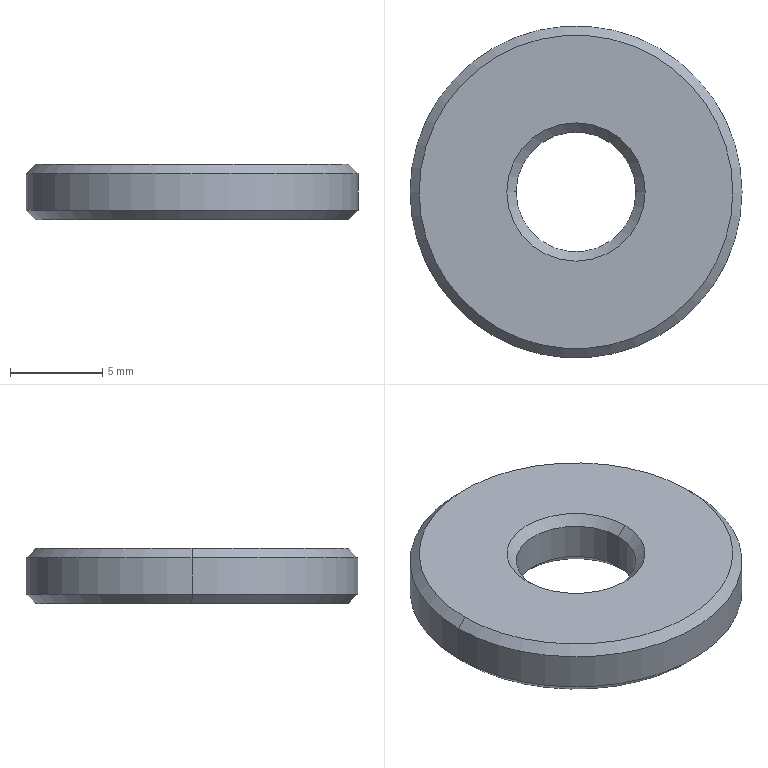Part | SolidWorks | features Chamfer 1, Extrusion 1 | 1 solid | 14 faces | box 18 x 18 x 3 mm | volume 644.616 mm3 | cone 8 | cylinder 4 | plane 2 | commonest cylinder face diameters 6.5 x2 18 x2
STEP:
#1=CARTESIAN_POINT('',(-3.25,0.,2.5));
#2=VERTEX_POINT('',#1);
#3=CARTESIAN_POINT('',(3.25,0.,2.5));
#4=VERTEX_POINT('',#3);
#5=CARTESIAN_POINT('',(0.,0.,2.5));
#6=DIRECTION('',(0.,0.,1.));
#7=DIRECTION('',(1.,0.,0.));
#8=AXIS2_PLACEMENT_3D('',#5,#6,#7);
#9=CIRCLE('',#8,3.25);
#10=EDGE_CURVE('',#2,#4,#9,.T.);
#11=ORIENTED_EDGE('',*,*,#10,.F.);
#12=CARTESIAN_POINT('',(-3.75,0.,3.));
#13=VERTEX_POINT('',#12);
#14=CARTESIAN_POINT('',(-3.25,0.,2.5));
#15=DIRECTION('',(-0.7071,0.,0.7071));
#16=VECTOR('',#15,1000.);
#17=LINE('',#14,#16);
#18=EDGE_CURVE('',#2,#13,#17,.T.);
#19=ORIENTED_EDGE('',*,*,#18,.T.);
#20=CARTESIAN_POINT('',(3.75,0.,3.));
#21=VERTEX_POINT('',#20);
#22=CARTESIAN_POINT('',(0.,0.,3.));
#23=DIRECTION('',(0.,0.,-1.));
#24=DIRECTION('',(1.,0.,0.));
#25=AXIS2_PLACEMENT_3D('',#22,#23,#24);
#26=CIRCLE('',#25,3.75);
#27=EDGE_CURVE('',#21,#13,#26,.T.);
#28=ORIENTED_EDGE('',*,*,#27,.F.);
#29=CARTESIAN_POINT('',(3.25,0.,2.5));
#30=DIRECTION('',(0.7071,0.,0.7071));
#31=VECTOR('',#30,1000.);
#32=LINE('',#29,#31);
#33=EDGE_CURVE('',#4,#21,#32,.T.);
#34=ORIENTED_EDGE('',*,*,#33,.F.);
#35=EDGE_LOOP('',(#11,#19,#28,#34));
#36=FACE_OUTER_BOUND('',#35,.T.);
#37=CARTESIAN_POINT('',(0.,0.,2.5));
#38=DIRECTION('',(0.,0.,1.));
#39=DIRECTION('',(1.,0.,0.));
#40=AXIS2_PLACEMENT_3D('',#37,#38,#39);
#41=CONICAL_SURFACE('',#40,3.25,0.7854);
#42=ADVANCED_FACE('',(#36),#41,.F.);
#43=CARTESIAN_POINT('',(3.25,0.,0.5));
#44=VERTEX_POINT('',#43);
#45=CARTESIAN_POINT('',(-3.25,0.,0.5));
#46=VERTEX_POINT('',#45);
#47=CARTESIAN_POINT('',(0.,0.,0.5));
#48=DIRECTION('',(0.,0.,-1.));
#49=DIRECTION('',(1.,0.,0.));
#50=AXIS2_PLACEMENT_3D('',#47,#48,#49);
#51=CIRCLE('',#50,3.25);
#52=EDGE_CURVE('',#44,#46,#51,.T.);
#53=ORIENTED_EDGE('',*,*,#52,.F.);
#54=CARTESIAN_POINT('',(3.75,0.,0.));
#55=VERTEX_POINT('',#54);
#56=CARTESIAN_POINT('',(3.75,0.,0.));
#57=DIRECTION('',(0.7071,0.,-0.7071));
#58=VECTOR('',#57,1000.);
#59=LINE('',#56,#58);
#60=EDGE_CURVE('',#44,#55,#59,.T.);
#61=ORIENTED_EDGE('',*,*,#60,.T.);
#62=CARTESIAN_POINT('',(-3.75,0.,0.));
#63=VERTEX_POINT('',#62);
#64=CARTESIAN_POINT('',(0.,0.,0.));
#65=DIRECTION('',(0.,0.,1.));
#66=DIRECTION('',(1.,0.,0.));
#67=AXIS2_PLACEMENT_3D('',#64,#65,#66);
#68=CIRCLE('',#67,3.75);
#69=EDGE_CURVE('',#63,#55,#68,.T.);
#70=ORIENTED_EDGE('',*,*,#69,.F.);
#71=CARTESIAN_POINT('',(-3.75,0.,0.));
#72=DIRECTION('',(-0.7071,0.,-0.7071));
#73=VECTOR('',#72,1000.);
#74=LINE('',#71,#73);
#75=EDGE_CURVE('',#46,#63,#74,.T.);
#76=ORIENTED_EDGE('',*,*,#75,.F.);
#77=EDGE_LOOP('',(#53,#61,#70,#76));
#78=FACE_OUTER_BOUND('',#77,.T.);
#79=CARTESIAN_POINT('',(0.,0.,0.));
#80=DIRECTION('',(0.,0.,-1.));
#81=DIRECTION('',(-1.,0.,0.));
#82=AXIS2_PLACEMENT_3D('',#79,#80,#81);
#83=CONICAL_SURFACE('',#82,3.75,0.7854);
#84=ADVANCED_FACE('',(#78),#83,.F.);
#85=CARTESIAN_POINT('',(8.5,0.,3.));
#86=VERTEX_POINT('',#85);
#87=CARTESIAN_POINT('',(-8.5,0.,3.));
#88=VERTEX_POINT('',#87);
#89=CARTESIAN_POINT('',(0.,0.,3.));
#90=DIRECTION('',(0.,0.,1.));
#91=DIRECTION('',(1.,0.,0.));
#92=AXIS2_PLACEMENT_3D('',#89,#90,#91);
#93=CIRCLE('',#92,8.5);
#94=EDGE_CURVE('',#86,#88,#93,.T.);
#95=ORIENTED_EDGE('',*,*,#94,.F.);
#96=CARTESIAN_POINT('',(9.,0.,2.5));
#97=VERTEX_POINT('',#96);
#98=CARTESIAN_POINT('',(8.5,0.,3.));
#99=DIRECTION('',(0.7071,0.,-0.7071));
#100=VECTOR('',#99,1000.);
#101=LINE('',#98,#100);
#102=EDGE_CURVE('',#86,#97,#101,.T.);
#103=ORIENTED_EDGE('',*,*,#102,.T.);
#104=CARTESIAN_POINT('',(-9.,0.,2.5));
#105=VERTEX_POINT('',#104);
#106=CARTESIAN_POINT('',(0.,0.,2.5));
#107=DIRECTION('',(0.,0.,-1.));
#108=DIRECTION('',(1.,0.,0.));
#109=AXIS2_PLACEMENT_3D('',#106,#107,#108);
#110=CIRCLE('',#109,9.);
#111=EDGE_CURVE('',#105,#97,#110,.T.);
#112=ORIENTED_EDGE('',*,*,#111,.F.);
#113=CARTESIAN_POINT('',(-8.5,0.,3.));
#114=DIRECTION('',(-0.7071,0.,-0.7071));
#115=VECTOR('',#114,1000.);
#116=LINE('',#113,#115);
#117=EDGE_CURVE('',#88,#105,#116,.T.);
#118=ORIENTED_EDGE('',*,*,#117,.F.);
#119=EDGE_LOOP('',(#95,#103,#112,#118));
#120=FACE_OUTER_BOUND('',#119,.T.);
#121=CARTESIAN_POINT('',(0.,0.,3.));
#122=DIRECTION('',(0.,0.,-1.));
#123=DIRECTION('',(-1.,0.,0.));
#124=AXIS2_PLACEMENT_3D('',#121,#122,#123);
#125=CONICAL_SURFACE('',#124,8.5,0.7854);
#126=ADVANCED_FACE('',(#120),#125,.T.);
#127=CARTESIAN_POINT('',(-8.5,0.,0.));
#128=VERTEX_POINT('',#127);
#129=CARTESIAN_POINT('',(8.5,0.,0.));
#130=VERTEX_POINT('',#129);
#131=CARTESIAN_POINT('',(0.,0.,0.));
#132=DIRECTION('',(0.,0.,-1.));
#133=DIRECTION('',(1.,0.,0.));
#134=AXIS2_PLACEMENT_3D('',#131,#132,#133);
#135=CIRCLE('',#134,8.5);
#136=EDGE_CURVE('',#128,#130,#135,.T.);
#137=ORIENTED_EDGE('',*,*,#136,.F.);
#138=CARTESIAN_POINT('',(-9.,0.,0.5));
#139=VERTEX_POINT('',#138);
#140=CARTESIAN_POINT('',(-9.,0.,0.5));
#141=DIRECTION('',(-0.7071,0.,0.7071));
#142=VECTOR('',#141,1000.);
#143=LINE('',#140,#142);
#144=EDGE_CURVE('',#128,#139,#143,.T.);
#145=ORIENTED_EDGE('',*,*,#144,.T.);
#146=CARTESIAN_POINT('',(9.,0.,0.5));
#147=VERTEX_POINT('',#146);
#148=CARTESIAN_POINT('',(0.,0.,0.5));
#149=DIRECTION('',(0.,0.,1.));
#150=DIRECTION('',(1.,0.,0.));
#151=AXIS2_PLACEMENT_3D('',#148,#149,#150);
#152=CIRCLE('',#151,9.);
#153=EDGE_CURVE('',#147,#139,#152,.T.);
#154=ORIENTED_EDGE('',*,*,#153,.F.);
#155=CARTESIAN_POINT('',(9.,0.,0.5));
#156=DIRECTION('',(0.7071,0.,0.7071));
#157=VECTOR('',#156,1000.);
#158=LINE('',#155,#157);
#159=EDGE_CURVE('',#130,#147,#158,.T.);
#160=ORIENTED_EDGE('',*,*,#159,.F.);
#161=EDGE_LOOP('',(#137,#145,#154,#160));
#162=FACE_OUTER_BOUND('',#161,.T.);
#163=CARTESIAN_POINT('',(0.,0.,0.5));
#164=DIRECTION('',(0.,0.,1.));
#165=DIRECTION('',(1.,0.,0.));
#166=AXIS2_PLACEMENT_3D('',#163,#164,#165);
#167=CONICAL_SURFACE('',#166,9.,0.7854);
#168=ADVANCED_FACE('',(#162),#167,.T.);
#169=ORIENTED_EDGE('',*,*,#10,.T.);
#170=CARTESIAN_POINT('',(3.25,0.,3.));
#171=DIRECTION('',(0.,0.,-1.));
#172=VECTOR('',#171,1000.);
#173=LINE('',#170,#172);
#174=EDGE_CURVE('',#4,#44,#173,.T.);
#175=ORIENTED_EDGE('',*,*,#174,.T.);
#176=ORIENTED_EDGE('',*,*,#52,.T.);
#177=CARTESIAN_POINT('',(-3.25,0.,3.));
#178=DIRECTION('',(0.,0.,-1.));
#179=VECTOR('',#178,1000.);
#180=LINE('',#177,#179);
#181=EDGE_CURVE('',#2,#46,#180,.T.);
#182=ORIENTED_EDGE('',*,*,#181,.F.);
#183=EDGE_LOOP('',(#169,#175,#176,#182));
#184=FACE_OUTER_BOUND('',#183,.T.);
#185=CARTESIAN_POINT('',(0.,0.,3.));
#186=DIRECTION('',(0.,0.,-1.));
#187=DIRECTION('',(-1.,0.,0.));
#188=AXIS2_PLACEMENT_3D('',#185,#186,#187);
#189=CYLINDRICAL_SURFACE('',#188,3.25);
#190=ADVANCED_FACE('',(#184),#189,.F.);
#191=ORIENTED_EDGE('',*,*,#111,.T.);
#192=CARTESIAN_POINT('',(9.,0.,3.));
#193=DIRECTION('',(0.,0.,-1.));
#194=VECTOR('',#193,1000.);
#195=LINE('',#192,#194);
#196=EDGE_CURVE('',#97,#147,#195,.T.);
#197=ORIENTED_EDGE('',*,*,#196,.T.);
#198=ORIENTED_EDGE('',*,*,#153,.T.);
#199=CARTESIAN_POINT('',(-9.,0.,3.));
#200=DIRECTION('',(0.,0.,-1.));
#201=VECTOR('',#200,1000.);
#202=LINE('',#199,#201);
#203=EDGE_CURVE('',#105,#139,#202,.T.);
#204=ORIENTED_EDGE('',*,*,#203,.F.);
#205=EDGE_LOOP('',(#191,#197,#198,#204));
#206=FACE_OUTER_BOUND('',#205,.T.);
#207=CARTESIAN_POINT('',(0.,0.,3.));
#208=DIRECTION('',(0.,0.,-1.));
#209=DIRECTION('',(-1.,0.,0.));
#210=AXIS2_PLACEMENT_3D('',#207,#208,#209);
#211=CYLINDRICAL_SURFACE('',#210,9.);
#212=ADVANCED_FACE('',(#206),#211,.T.);
#213=CARTESIAN_POINT('',(0.,0.,3.));
#214=DIRECTION('',(0.,0.,1.));
#215=DIRECTION('',(1.,0.,0.));
#216=AXIS2_PLACEMENT_3D('',#213,#214,#215);
#217=CIRCLE('',#216,8.5);
#218=EDGE_CURVE('',#88,#86,#217,.T.);
#219=ORIENTED_EDGE('',*,*,#218,.T.);
#220=ORIENTED_EDGE('',*,*,#94,.T.);
#221=EDGE_LOOP('',(#219,#220));
#222=FACE_OUTER_BOUND('',#221,.T.);
#223=ORIENTED_EDGE('',*,*,#27,.T.);
#224=CARTESIAN_POINT('',(0.,0.,3.));
#225=DIRECTION('',(0.,0.,-1.));
#226=DIRECTION('',(1.,0.,0.));
#227=AXIS2_PLACEMENT_3D('',#224,#225,#226);
#228=CIRCLE('',#227,3.75);
#229=EDGE_CURVE('',#13,#21,#228,.T.);
#230=ORIENTED_EDGE('',*,*,#229,.T.);
#231=EDGE_LOOP('',(#223,#230));
#232=FACE_BOUND('',#231,.T.);
#233=CARTESIAN_POINT('',(0.,0.,3.));
#234=DIRECTION('',(0.,0.,1.));
#235=DIRECTION('',(1.,0.,0.));
#236=AXIS2_PLACEMENT_3D('',#233,#234,#235);
#237=PLANE('',#236);
#238=ADVANCED_FACE('',(#222,#232),#237,.T.);
#239=CARTESIAN_POINT('',(0.,0.,0.));
#240=DIRECTION('',(0.,0.,-1.));
#241=DIRECTION('',(1.,0.,0.));
#242=AXIS2_PLACEMENT_3D('',#239,#240,#241);
#243=CIRCLE('',#242,8.5);
#244=EDGE_CURVE('',#130,#128,#243,.T.);
#245=ORIENTED_EDGE('',*,*,#244,.T.);
#246=ORIENTED_EDGE('',*,*,#136,.T.);
#247=EDGE_LOOP('',(#245,#246));
#248=FACE_OUTER_BOUND('',#247,.T.);
#249=ORIENTED_EDGE('',*,*,#69,.T.);
#250=CARTESIAN_POINT('',(0.,0.,0.));
#251=DIRECTION('',(0.,0.,1.));
#252=DIRECTION('',(1.,0.,0.));
#253=AXIS2_PLACEMENT_3D('',#250,#251,#252);
#254=CIRCLE('',#253,3.75);
#255=EDGE_CURVE('',#55,#63,#254,.T.);
#256=ORIENTED_EDGE('',*,*,#255,.T.);
#257=EDGE_LOOP('',(#249,#256));
#258=FACE_BOUND('',#257,.T.);
#259=CARTESIAN_POINT('',(0.,0.,0.));
#260=DIRECTION('',(0.,0.,1.));
#261=DIRECTION('',(1.,0.,0.));
#262=AXIS2_PLACEMENT_3D('',#259,#260,#261);
#263=PLANE('',#262);
#264=ADVANCED_FACE('',(#248,#258),#263,.F.);
#265=ORIENTED_EDGE('',*,*,#196,.F.);
#266=CARTESIAN_POINT('',(0.,0.,2.5));
#267=DIRECTION('',(0.,0.,-1.));
#268=DIRECTION('',(1.,0.,0.));
#269=AXIS2_PLACEMENT_3D('',#266,#267,#268);
#270=CIRCLE('',#269,9.);
#271=EDGE_CURVE('',#97,#105,#270,.T.);
#272=ORIENTED_EDGE('',*,*,#271,.T.);
#273=ORIENTED_EDGE('',*,*,#203,.T.);
#274=CARTESIAN_POINT('',(0.,0.,0.5));
#275=DIRECTION('',(0.,0.,1.));
#276=DIRECTION('',(1.,0.,0.));
#277=AXIS2_PLACEMENT_3D('',#274,#275,#276);
#278=CIRCLE('',#277,9.);
#279=EDGE_CURVE('',#139,#147,#278,.T.);
#280=ORIENTED_EDGE('',*,*,#279,.T.);
#281=EDGE_LOOP('',(#265,#272,#273,#280));
#282=FACE_OUTER_BOUND('',#281,.T.);
#283=CARTESIAN_POINT('',(0.,0.,3.));
#284=DIRECTION('',(0.,0.,-1.));
#285=DIRECTION('',(-1.,0.,0.));
#286=AXIS2_PLACEMENT_3D('',#283,#284,#285);
#287=CYLINDRICAL_SURFACE('',#286,9.);
#288=ADVANCED_FACE('',(#282),#287,.T.);
#289=ORIENTED_EDGE('',*,*,#174,.F.);
#290=CARTESIAN_POINT('',(0.,0.,2.5));
#291=DIRECTION('',(0.,0.,1.));
#292=DIRECTION('',(1.,0.,0.));
#293=AXIS2_PLACEMENT_3D('',#290,#291,#292);
#294=CIRCLE('',#293,3.25);
#295=EDGE_CURVE('',#4,#2,#294,.T.);
#296=ORIENTED_EDGE('',*,*,#295,.T.);
#297=ORIENTED_EDGE('',*,*,#181,.T.);
#298=CARTESIAN_POINT('',(0.,0.,0.5));
#299=DIRECTION('',(0.,0.,-1.));
#300=DIRECTION('',(1.,0.,0.));
#301=AXIS2_PLACEMENT_3D('',#298,#299,#300);
#302=CIRCLE('',#301,3.25);
#303=EDGE_CURVE('',#46,#44,#302,.T.);
#304=ORIENTED_EDGE('',*,*,#303,.T.);
#305=EDGE_LOOP('',(#289,#296,#297,#304));
#306=FACE_OUTER_BOUND('',#305,.T.);
#307=CARTESIAN_POINT('',(0.,0.,3.));
#308=DIRECTION('',(0.,0.,-1.));
#309=DIRECTION('',(-1.,0.,0.));
#310=AXIS2_PLACEMENT_3D('',#307,#308,#309);
#311=CYLINDRICAL_SURFACE('',#310,3.25);
#312=ADVANCED_FACE('',(#306),#311,.F.);
#313=ORIENTED_EDGE('',*,*,#144,.F.);
#314=ORIENTED_EDGE('',*,*,#244,.F.);
#315=ORIENTED_EDGE('',*,*,#159,.T.);
#316=ORIENTED_EDGE('',*,*,#279,.F.);
#317=EDGE_LOOP('',(#313,#314,#315,#316));
#318=FACE_OUTER_BOUND('',#317,.T.);
#319=CARTESIAN_POINT('',(0.,0.,0.5));
#320=DIRECTION('',(0.,0.,1.));
#321=DIRECTION('',(1.,0.,0.));
#322=AXIS2_PLACEMENT_3D('',#319,#320,#321);
#323=CONICAL_SURFACE('',#322,9.,0.7854);
#324=ADVANCED_FACE('',(#318),#323,.T.);
#325=ORIENTED_EDGE('',*,*,#102,.F.);
#326=ORIENTED_EDGE('',*,*,#218,.F.);
#327=ORIENTED_EDGE('',*,*,#117,.T.);
#328=ORIENTED_EDGE('',*,*,#271,.F.);
#329=EDGE_LOOP('',(#325,#326,#327,#328));
#330=FACE_OUTER_BOUND('',#329,.T.);
#331=CARTESIAN_POINT('',(0.,0.,3.));
#332=DIRECTION('',(0.,0.,-1.));
#333=DIRECTION('',(-1.,0.,0.));
#334=AXIS2_PLACEMENT_3D('',#331,#332,#333);
#335=CONICAL_SURFACE('',#334,8.5,0.7854);
#336=ADVANCED_FACE('',(#330),#335,.T.);
#337=ORIENTED_EDGE('',*,*,#60,.F.);
#338=ORIENTED_EDGE('',*,*,#303,.F.);
#339=ORIENTED_EDGE('',*,*,#75,.T.);
#340=ORIENTED_EDGE('',*,*,#255,.F.);
#341=EDGE_LOOP('',(#337,#338,#339,#340));
#342=FACE_OUTER_BOUND('',#341,.T.);
#343=CARTESIAN_POINT('',(0.,0.,0.));
#344=DIRECTION('',(0.,0.,-1.));
#345=DIRECTION('',(-1.,0.,0.));
#346=AXIS2_PLACEMENT_3D('',#343,#344,#345);
#347=CONICAL_SURFACE('',#346,3.75,0.7854);
#348=ADVANCED_FACE('',(#342),#347,.F.);
#349=ORIENTED_EDGE('',*,*,#18,.F.);
#350=ORIENTED_EDGE('',*,*,#295,.F.);
#351=ORIENTED_EDGE('',*,*,#33,.T.);
#352=ORIENTED_EDGE('',*,*,#229,.F.);
#353=EDGE_LOOP('',(#349,#350,#351,#352));
#354=FACE_OUTER_BOUND('',#353,.T.);
#355=CARTESIAN_POINT('',(0.,0.,2.5));
#356=DIRECTION('',(0.,0.,1.));
#357=DIRECTION('',(1.,0.,0.));
#358=AXIS2_PLACEMENT_3D('',#355,#356,#357);
#359=CONICAL_SURFACE('',#358,3.25,0.7854);
#360=ADVANCED_FACE('',(#354),#359,.F.);
#361=CLOSED_SHELL('',(#42,#84,#126,#168,#190,#212,#238,#264,#288,#312,#324,#336,#348,#360));
#362=MANIFOLD_SOLID_BREP('',#361);
#363=CARTESIAN_POINT('',(0.,0.,0.));
#364=DIRECTION('',(0.,0.,1.));
#365=DIRECTION('',(1.,0.,0.));
#366=AXIS2_PLACEMENT_3D('',#363,#364,#365);
#367=(LENGTH_UNIT()NAMED_UNIT(*)SI_UNIT(.MILLI.,.METRE.));
#368=UNCERTAINTY_MEASURE_WITH_UNIT(LENGTH_MEASURE(0.00001),#367,'','');
#369=(NAMED_UNIT(*)PLANE_ANGLE_UNIT()SI_UNIT($,.RADIAN.));
#370=(NAMED_UNIT(*)SI_UNIT($,.STERADIAN.)SOLID_ANGLE_UNIT());
#371=(GEOMETRIC_REPRESENTATION_CONTEXT(3)GLOBAL_UNCERTAINTY_ASSIGNED_CONTEXT((#368))GLOBAL_UNIT_ASSIGNED_CONTEXT((#367,#369,#370))REPRESENTATION_CONTEXT('',''));
#372=ADVANCED_BREP_SHAPE_REPRESENTATION('',(#362,#366),#371);